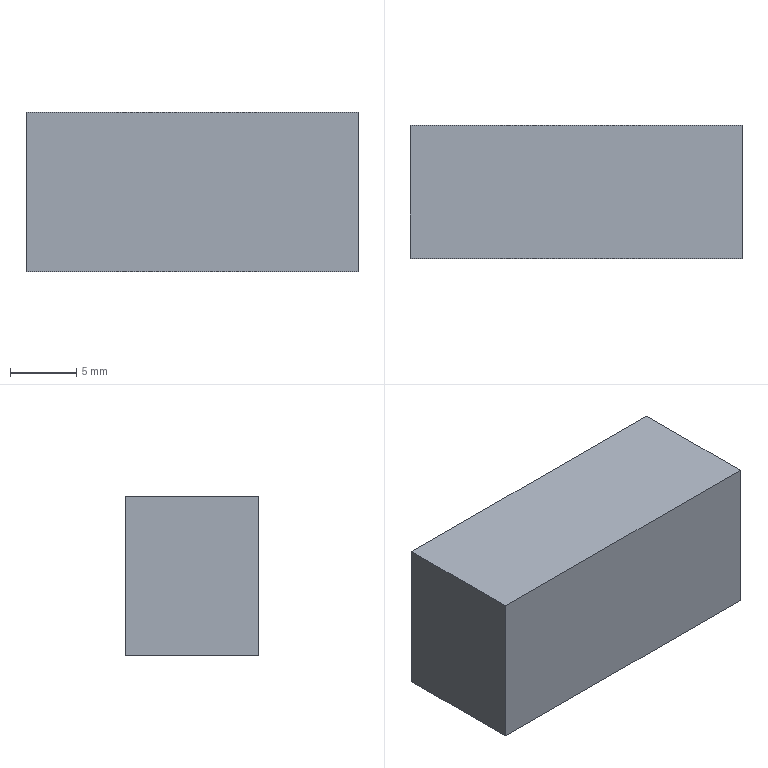Part | SolidWorks | features Extrusion 1 | 1 solid | 6 faces | box 25 x 10 x 12 mm | volume 3000 mm3 | plane 6
STEP:
#1=CARTESIAN_POINT('',(-12.5,5.,6.));
#2=VERTEX_POINT('',#1);
#3=CARTESIAN_POINT('',(-12.5,-5.,6.));
#4=VERTEX_POINT('',#3);
#5=CARTESIAN_POINT('',(-12.5,5.,6.));
#6=DIRECTION('',(0.,-1.,0.));
#7=VECTOR('',#6,1000.);
#8=LINE('',#5,#7);
#9=EDGE_CURVE('',#2,#4,#8,.T.);
#10=ORIENTED_EDGE('',*,*,#9,.F.);
#11=CARTESIAN_POINT('',(-12.5,5.,-6.));
#12=VERTEX_POINT('',#11);
#13=CARTESIAN_POINT('',(-12.5,5.,-6.));
#14=DIRECTION('',(0.,0.,1.));
#15=VECTOR('',#14,1000.);
#16=LINE('',#13,#15);
#17=EDGE_CURVE('',#12,#2,#16,.T.);
#18=ORIENTED_EDGE('',*,*,#17,.F.);
#19=CARTESIAN_POINT('',(-12.5,-5.,-6.));
#20=VERTEX_POINT('',#19);
#21=CARTESIAN_POINT('',(-12.5,5.,-6.));
#22=DIRECTION('',(0.,-1.,0.));
#23=VECTOR('',#22,1000.);
#24=LINE('',#21,#23);
#25=EDGE_CURVE('',#12,#20,#24,.T.);
#26=ORIENTED_EDGE('',*,*,#25,.T.);
#27=CARTESIAN_POINT('',(-12.5,-5.,-6.));
#28=DIRECTION('',(0.,0.,1.));
#29=VECTOR('',#28,1000.);
#30=LINE('',#27,#29);
#31=EDGE_CURVE('',#20,#4,#30,.T.);
#32=ORIENTED_EDGE('',*,*,#31,.T.);
#33=EDGE_LOOP('',(#10,#18,#26,#32));
#34=FACE_OUTER_BOUND('',#33,.T.);
#35=CARTESIAN_POINT('',(-12.5,5.,-6.));
#36=DIRECTION('',(-1.,0.,0.));
#37=DIRECTION('',(0.,0.,1.));
#38=AXIS2_PLACEMENT_3D('',#35,#36,#37);
#39=PLANE('',#38);
#40=ADVANCED_FACE('',(#34),#39,.T.);
#41=CARTESIAN_POINT('',(12.5,5.,6.));
#42=VERTEX_POINT('',#41);
#43=CARTESIAN_POINT('',(12.5,5.,6.));
#44=DIRECTION('',(-1.,0.,0.));
#45=VECTOR('',#44,1000.);
#46=LINE('',#43,#45);
#47=EDGE_CURVE('',#42,#2,#46,.T.);
#48=ORIENTED_EDGE('',*,*,#47,.F.);
#49=CARTESIAN_POINT('',(12.5,5.,-6.));
#50=VERTEX_POINT('',#49);
#51=CARTESIAN_POINT('',(12.5,5.,-6.));
#52=DIRECTION('',(0.,0.,1.));
#53=VECTOR('',#52,1000.);
#54=LINE('',#51,#53);
#55=EDGE_CURVE('',#50,#42,#54,.T.);
#56=ORIENTED_EDGE('',*,*,#55,.F.);
#57=CARTESIAN_POINT('',(12.5,5.,-6.));
#58=DIRECTION('',(-1.,0.,0.));
#59=VECTOR('',#58,1000.);
#60=LINE('',#57,#59);
#61=EDGE_CURVE('',#50,#12,#60,.T.);
#62=ORIENTED_EDGE('',*,*,#61,.T.);
#63=ORIENTED_EDGE('',*,*,#17,.T.);
#64=EDGE_LOOP('',(#48,#56,#62,#63));
#65=FACE_OUTER_BOUND('',#64,.T.);
#66=CARTESIAN_POINT('',(12.5,5.,-6.));
#67=DIRECTION('',(0.,1.,0.));
#68=DIRECTION('',(0.,0.,1.));
#69=AXIS2_PLACEMENT_3D('',#66,#67,#68);
#70=PLANE('',#69);
#71=ADVANCED_FACE('',(#65),#70,.T.);
#72=CARTESIAN_POINT('',(12.5,-5.,6.));
#73=VERTEX_POINT('',#72);
#74=CARTESIAN_POINT('',(12.5,-5.,6.));
#75=DIRECTION('',(0.,1.,0.));
#76=VECTOR('',#75,1000.);
#77=LINE('',#74,#76);
#78=EDGE_CURVE('',#73,#42,#77,.T.);
#79=ORIENTED_EDGE('',*,*,#78,.F.);
#80=CARTESIAN_POINT('',(12.5,-5.,-6.));
#81=VERTEX_POINT('',#80);
#82=CARTESIAN_POINT('',(12.5,-5.,-6.));
#83=DIRECTION('',(0.,0.,1.));
#84=VECTOR('',#83,1000.);
#85=LINE('',#82,#84);
#86=EDGE_CURVE('',#81,#73,#85,.T.);
#87=ORIENTED_EDGE('',*,*,#86,.F.);
#88=CARTESIAN_POINT('',(12.5,-5.,-6.));
#89=DIRECTION('',(0.,1.,0.));
#90=VECTOR('',#89,1000.);
#91=LINE('',#88,#90);
#92=EDGE_CURVE('',#81,#50,#91,.T.);
#93=ORIENTED_EDGE('',*,*,#92,.T.);
#94=ORIENTED_EDGE('',*,*,#55,.T.);
#95=EDGE_LOOP('',(#79,#87,#93,#94));
#96=FACE_OUTER_BOUND('',#95,.T.);
#97=CARTESIAN_POINT('',(12.5,-5.,-6.));
#98=DIRECTION('',(1.,0.,0.));
#99=DIRECTION('',(0.,0.,-1.));
#100=AXIS2_PLACEMENT_3D('',#97,#98,#99);
#101=PLANE('',#100);
#102=ADVANCED_FACE('',(#96),#101,.T.);
#103=CARTESIAN_POINT('',(-12.5,-5.,6.));
#104=DIRECTION('',(1.,0.,0.));
#105=VECTOR('',#104,1000.);
#106=LINE('',#103,#105);
#107=EDGE_CURVE('',#4,#73,#106,.T.);
#108=ORIENTED_EDGE('',*,*,#107,.F.);
#109=ORIENTED_EDGE('',*,*,#31,.F.);
#110=CARTESIAN_POINT('',(-12.5,-5.,-6.));
#111=DIRECTION('',(1.,0.,0.));
#112=VECTOR('',#111,1000.);
#113=LINE('',#110,#112);
#114=EDGE_CURVE('',#20,#81,#113,.T.);
#115=ORIENTED_EDGE('',*,*,#114,.T.);
#116=ORIENTED_EDGE('',*,*,#86,.T.);
#117=EDGE_LOOP('',(#108,#109,#115,#116));
#118=FACE_OUTER_BOUND('',#117,.T.);
#119=CARTESIAN_POINT('',(-12.5,-5.,-6.));
#120=DIRECTION('',(0.,-1.,0.));
#121=DIRECTION('',(0.,0.,-1.));
#122=AXIS2_PLACEMENT_3D('',#119,#120,#121);
#123=PLANE('',#122);
#124=ADVANCED_FACE('',(#118),#123,.T.);
#125=ORIENTED_EDGE('',*,*,#25,.F.);
#126=ORIENTED_EDGE('',*,*,#61,.F.);
#127=ORIENTED_EDGE('',*,*,#92,.F.);
#128=ORIENTED_EDGE('',*,*,#114,.F.);
#129=EDGE_LOOP('',(#125,#126,#127,#128));
#130=FACE_OUTER_BOUND('',#129,.T.);
#131=CARTESIAN_POINT('',(0.,0.,-6.));
#132=DIRECTION('',(0.,0.,1.));
#133=DIRECTION('',(1.,0.,0.));
#134=AXIS2_PLACEMENT_3D('',#131,#132,#133);
#135=PLANE('',#134);
#136=ADVANCED_FACE('',(#130),#135,.F.);
#137=ORIENTED_EDGE('',*,*,#9,.T.);
#138=ORIENTED_EDGE('',*,*,#107,.T.);
#139=ORIENTED_EDGE('',*,*,#78,.T.);
#140=ORIENTED_EDGE('',*,*,#47,.T.);
#141=EDGE_LOOP('',(#137,#138,#139,#140));
#142=FACE_OUTER_BOUND('',#141,.T.);
#143=CARTESIAN_POINT('',(0.,0.,6.));
#144=DIRECTION('',(0.,0.,1.));
#145=DIRECTION('',(1.,0.,0.));
#146=AXIS2_PLACEMENT_3D('',#143,#144,#145);
#147=PLANE('',#146);
#148=ADVANCED_FACE('',(#142),#147,.T.);
#149=CLOSED_SHELL('',(#40,#71,#102,#124,#136,#148));
#150=MANIFOLD_SOLID_BREP('',#149);
#151=CARTESIAN_POINT('',(0.,0.,0.));
#152=DIRECTION('',(0.,0.,1.));
#153=DIRECTION('',(1.,0.,0.));
#154=AXIS2_PLACEMENT_3D('',#151,#152,#153);
#155=(LENGTH_UNIT()NAMED_UNIT(*)SI_UNIT(.MILLI.,.METRE.));
#156=UNCERTAINTY_MEASURE_WITH_UNIT(LENGTH_MEASURE(0.00001),#155,'','');
#157=(NAMED_UNIT(*)PLANE_ANGLE_UNIT()SI_UNIT($,.RADIAN.));
#158=(NAMED_UNIT(*)SI_UNIT($,.STERADIAN.)SOLID_ANGLE_UNIT());
#159=(GEOMETRIC_REPRESENTATION_CONTEXT(3)GLOBAL_UNCERTAINTY_ASSIGNED_CONTEXT((#156))GLOBAL_UNIT_ASSIGNED_CONTEXT((#155,#157,#158))REPRESENTATION_CONTEXT('',''));
#160=ADVANCED_BREP_SHAPE_REPRESENTATION('',(#150,#154),#159);